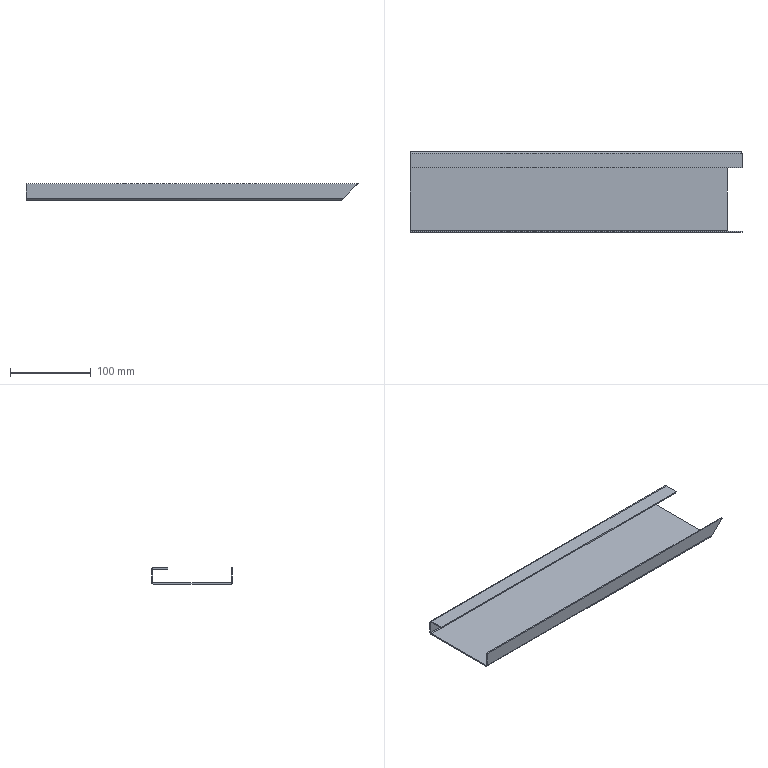Part | STEP file | 护栏90度踢脚Plate-1 | 1 solid | 18 faces | box 410 x 100 x 20 mm | volume 90870 mm3 | plane 12 | cylinder 6 | commonest cylinder face diameters 2 x3 5 x3